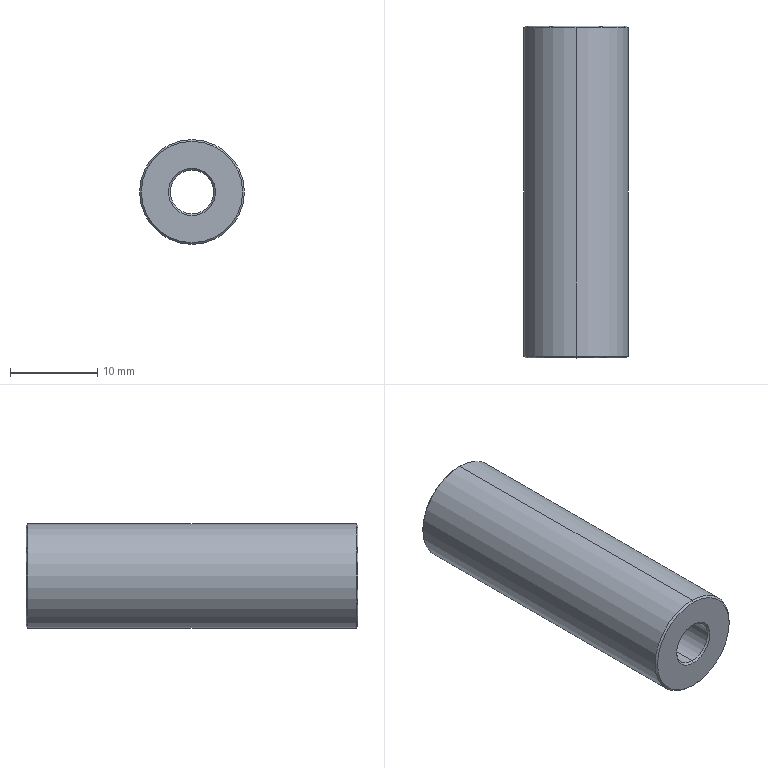Part | STEP file | NCLA5-12-38 | 1 solid | 14 faces | box 12 x 38 x 12 mm | volume 3549 mm3 | cone 8 | cylinder 4 | plane 2 | commonest cylinder face diameters 5 x2 12 x2
STEP:
#1=CARTESIAN_POINT('',(0.,0.,0.));
#2=DIRECTION('',(0.,0.,1.));
#3=DIRECTION('',(1.,0.,0.));
#4=AXIS2_PLACEMENT_3D('',#1,#2,#3);
#5=CARTESIAN_POINT('',(0.,0.2,-2.5));
#6=VERTEX_POINT('',#5);
#7=CARTESIAN_POINT('',(0.,0.,-2.7));
#8=VERTEX_POINT('',#7);
#9=CARTESIAN_POINT('',(0.,0.2,-2.5));
#10=DIRECTION('',(0.,-0.7071,-0.7071));
#11=VECTOR('',#10,1.);
#12=LINE('',#9,#11);
#13=CARTESIAN_POINT('',(0.,0.2,0.));
#14=DIRECTION('',(0.,-1.,0.));
#15=DIRECTION('',(0.,0.,-1.));
#16=AXIS2_PLACEMENT_3D('',#13,#14,#15);
#17=CONICAL_SURFACE('',#16,2.5,0.7854);
#18=CARTESIAN_POINT('',(6.283,0.));
#19=DIRECTION('',(0.,1.));
#20=VECTOR('',#19,1.);
#21=LINE('',#18,#20);
#22=(GEOMETRIC_REPRESENTATION_CONTEXT(2)PARAMETRIC_REPRESENTATION_CONTEXT()REPRESENTATION_CONTEXT('',''));
#23=DEFINITIONAL_REPRESENTATION('',(#21),#22);
#24=PCURVE('',#17,#23);
#25=CARTESIAN_POINT('',(0.,0.2,0.));
#26=DIRECTION('',(0.,-1.,0.));
#27=DIRECTION('',(0.,0.,-1.));
#28=AXIS2_PLACEMENT_3D('',#25,#26,#27);
#29=CONICAL_SURFACE('',#28,2.5,0.7854);
#30=CARTESIAN_POINT('',(0.,0.));
#31=DIRECTION('',(0.,1.));
#32=VECTOR('',#31,1.);
#33=LINE('',#30,#32);
#34=(GEOMETRIC_REPRESENTATION_CONTEXT(2)PARAMETRIC_REPRESENTATION_CONTEXT()REPRESENTATION_CONTEXT('',''));
#35=DEFINITIONAL_REPRESENTATION('',(#33),#34);
#36=PCURVE('',#29,#35);
#37=SURFACE_CURVE('',#12,(#24,#36),.PCURVE_S1.);
#38=EDGE_CURVE('',#6,#8,#37,.T.);
#39=ORIENTED_EDGE('',*,*,#38,.T.);
#40=CARTESIAN_POINT('',(0.,0.,2.7));
#41=VERTEX_POINT('',#40);
#42=CARTESIAN_POINT('',(0.,0.,0.));
#43=DIRECTION('',(0.,-1.,0.));
#44=DIRECTION('',(0.,0.,-1.));
#45=AXIS2_PLACEMENT_3D('',#42,#43,#44);
#46=CIRCLE('',#45,2.7);
#47=CARTESIAN_POINT('',(0.,0.2));
#48=DIRECTION('',(1.,0.));
#49=VECTOR('',#48,1.);
#50=LINE('',#47,#49);
#51=(GEOMETRIC_REPRESENTATION_CONTEXT(2)PARAMETRIC_REPRESENTATION_CONTEXT()REPRESENTATION_CONTEXT('',''));
#52=DEFINITIONAL_REPRESENTATION('',(#50),#51);
#53=PCURVE('',#17,#52);
#54=CARTESIAN_POINT('',(7.3,0.,0.));
#55=DIRECTION('',(0.,1.,0.));
#56=DIRECTION('',(0.,0.,1.));
#57=AXIS2_PLACEMENT_3D('',#54,#55,#56);
#58=PLANE('',#57);
#59=CARTESIAN_POINT('',(-2.7,-7.3));
#60=CARTESIAN_POINT('',(-2.7,-2.623));
#61=CARTESIAN_POINT('',(1.35,-4.962));
#62=CARTESIAN_POINT('',(5.4,-7.3));
#63=CARTESIAN_POINT('',(1.35,-9.638));
#64=CARTESIAN_POINT('',(-2.7,-11.977));
#65=CARTESIAN_POINT('',(-2.7,-7.3));
#66=(BOUNDED_CURVE()B_SPLINE_CURVE(2,(#59,#60,#61,#62,#63,#64,#65),.UNSPECIFIED.,.T.,.F.)B_SPLINE_CURVE_WITH_KNOTS((1,2,2,2,2,1),(-2.094,0.,2.094,4.189,6.283,8.378),.UNSPECIFIED.)CURVE()GEOMETRIC_REPRESENTATION_ITEM()RATIONAL_B_SPLINE_CURVE((1.,0.5,1.,0.5,1.,0.5,1.))REPRESENTATION_ITEM(''));
#67=(GEOMETRIC_REPRESENTATION_CONTEXT(2)PARAMETRIC_REPRESENTATION_CONTEXT()REPRESENTATION_CONTEXT('',''));
#68=DEFINITIONAL_REPRESENTATION('',(#66),#67);
#69=PCURVE('',#58,#68);
#70=SURFACE_CURVE('',#46,(#53,#69),.PCURVE_S1.);
#71=EDGE_CURVE('',#41,#8,#70,.T.);
#72=ORIENTED_EDGE('',*,*,#71,.F.);
#73=CARTESIAN_POINT('',(0.,0.2,2.5));
#74=VERTEX_POINT('',#73);
#75=CARTESIAN_POINT('',(0.,0.2,2.5));
#76=DIRECTION('',(0.,-0.7071,0.7071));
#77=VECTOR('',#76,1.);
#78=LINE('',#75,#77);
#79=CARTESIAN_POINT('',(3.142,0.));
#80=DIRECTION('',(0.,1.));
#81=VECTOR('',#80,1.);
#82=LINE('',#79,#81);
#83=(GEOMETRIC_REPRESENTATION_CONTEXT(2)PARAMETRIC_REPRESENTATION_CONTEXT()REPRESENTATION_CONTEXT('',''));
#84=DEFINITIONAL_REPRESENTATION('',(#82),#83);
#85=PCURVE('',#17,#84);
#86=CARTESIAN_POINT('',(3.142,0.));
#87=DIRECTION('',(0.,1.));
#88=VECTOR('',#87,1.);
#89=LINE('',#86,#88);
#90=(GEOMETRIC_REPRESENTATION_CONTEXT(2)PARAMETRIC_REPRESENTATION_CONTEXT()REPRESENTATION_CONTEXT('',''));
#91=DEFINITIONAL_REPRESENTATION('',(#89),#90);
#92=PCURVE('',#29,#91);
#93=SURFACE_CURVE('',#78,(#85,#92),.PCURVE_S1.);
#94=EDGE_CURVE('',#74,#41,#93,.T.);
#95=ORIENTED_EDGE('',*,*,#94,.F.);
#96=CARTESIAN_POINT('',(0.,0.2,0.));
#97=DIRECTION('',(0.,-1.,0.));
#98=DIRECTION('',(0.,0.,-1.));
#99=AXIS2_PLACEMENT_3D('',#96,#97,#98);
#100=CIRCLE('',#99,2.5);
#101=CARTESIAN_POINT('',(0.,0.));
#102=DIRECTION('',(1.,0.));
#103=VECTOR('',#102,1.);
#104=LINE('',#101,#103);
#105=(GEOMETRIC_REPRESENTATION_CONTEXT(2)PARAMETRIC_REPRESENTATION_CONTEXT()REPRESENTATION_CONTEXT('',''));
#106=DEFINITIONAL_REPRESENTATION('',(#104),#105);
#107=PCURVE('',#17,#106);
#108=CARTESIAN_POINT('',(0.,0.,0.));
#109=DIRECTION('',(0.,-1.,0.));
#110=DIRECTION('',(0.,0.,-1.));
#111=AXIS2_PLACEMENT_3D('',#108,#109,#110);
#112=CYLINDRICAL_SURFACE('',#111,2.5);
#113=CARTESIAN_POINT('',(0.,-0.2));
#114=DIRECTION('',(1.,0.));
#115=VECTOR('',#114,1.);
#116=LINE('',#113,#115);
#117=(GEOMETRIC_REPRESENTATION_CONTEXT(2)PARAMETRIC_REPRESENTATION_CONTEXT()REPRESENTATION_CONTEXT('',''));
#118=DEFINITIONAL_REPRESENTATION('',(#116),#117);
#119=PCURVE('',#112,#118);
#120=SURFACE_CURVE('',#100,(#107,#119),.PCURVE_S1.);
#121=EDGE_CURVE('',#74,#6,#120,.T.);
#122=ORIENTED_EDGE('',*,*,#121,.T.);
#123=EDGE_LOOP('',(#39,#72,#95,#122));
#124=FACE_BOUND('',#123,.F.);
#125=ADVANCED_FACE('',(#124),#17,.F.);
#126=CARTESIAN_POINT('',(0.,37.8,-2.5));
#127=VERTEX_POINT('',#126);
#128=CARTESIAN_POINT('',(0.,0.,-2.5));
#129=DIRECTION('',(0.,-1.,0.));
#130=VECTOR('',#129,1.);
#131=LINE('',#128,#130);
#132=CARTESIAN_POINT('',(6.283,0.));
#133=DIRECTION('',(0.,1.));
#134=VECTOR('',#133,1.);
#135=LINE('',#132,#134);
#136=(GEOMETRIC_REPRESENTATION_CONTEXT(2)PARAMETRIC_REPRESENTATION_CONTEXT()REPRESENTATION_CONTEXT('',''));
#137=DEFINITIONAL_REPRESENTATION('',(#135),#136);
#138=PCURVE('',#112,#137);
#139=CARTESIAN_POINT('',(0.,0.,0.));
#140=DIRECTION('',(0.,-1.,0.));
#141=DIRECTION('',(0.,0.,-1.));
#142=AXIS2_PLACEMENT_3D('',#139,#140,#141);
#143=CYLINDRICAL_SURFACE('',#142,2.5);
#144=CARTESIAN_POINT('',(0.,0.));
#145=DIRECTION('',(0.,1.));
#146=VECTOR('',#145,1.);
#147=LINE('',#144,#146);
#148=(GEOMETRIC_REPRESENTATION_CONTEXT(2)PARAMETRIC_REPRESENTATION_CONTEXT()REPRESENTATION_CONTEXT('',''));
#149=DEFINITIONAL_REPRESENTATION('',(#147),#148);
#150=PCURVE('',#143,#149);
#151=SURFACE_CURVE('',#131,(#138,#150),.PCURVE_S1.);
#152=EDGE_CURVE('',#127,#6,#151,.T.);
#153=ORIENTED_EDGE('',*,*,#152,.T.);
#154=ORIENTED_EDGE('',*,*,#121,.F.);
#155=CARTESIAN_POINT('',(0.,37.8,2.5));
#156=VERTEX_POINT('',#155);
#157=CARTESIAN_POINT('',(0.,0.,2.5));
#158=DIRECTION('',(0.,-1.,0.));
#159=VECTOR('',#158,1.);
#160=LINE('',#157,#159);
#161=CARTESIAN_POINT('',(3.142,0.));
#162=DIRECTION('',(0.,1.));
#163=VECTOR('',#162,1.);
#164=LINE('',#161,#163);
#165=(GEOMETRIC_REPRESENTATION_CONTEXT(2)PARAMETRIC_REPRESENTATION_CONTEXT()REPRESENTATION_CONTEXT('',''));
#166=DEFINITIONAL_REPRESENTATION('',(#164),#165);
#167=PCURVE('',#112,#166);
#168=CARTESIAN_POINT('',(3.142,0.));
#169=DIRECTION('',(0.,1.));
#170=VECTOR('',#169,1.);
#171=LINE('',#168,#170);
#172=(GEOMETRIC_REPRESENTATION_CONTEXT(2)PARAMETRIC_REPRESENTATION_CONTEXT()REPRESENTATION_CONTEXT('',''));
#173=DEFINITIONAL_REPRESENTATION('',(#171),#172);
#174=PCURVE('',#143,#173);
#175=SURFACE_CURVE('',#160,(#167,#174),.PCURVE_S1.);
#176=EDGE_CURVE('',#156,#74,#175,.T.);
#177=ORIENTED_EDGE('',*,*,#176,.F.);
#178=CARTESIAN_POINT('',(0.,37.8,0.));
#179=DIRECTION('',(0.,-1.,0.));
#180=DIRECTION('',(0.,0.,-1.));
#181=AXIS2_PLACEMENT_3D('',#178,#179,#180);
#182=CIRCLE('',#181,2.5);
#183=CARTESIAN_POINT('',(0.,-37.8));
#184=DIRECTION('',(1.,0.));
#185=VECTOR('',#184,1.);
#186=LINE('',#183,#185);
#187=(GEOMETRIC_REPRESENTATION_CONTEXT(2)PARAMETRIC_REPRESENTATION_CONTEXT()REPRESENTATION_CONTEXT('',''));
#188=DEFINITIONAL_REPRESENTATION('',(#186),#187);
#189=PCURVE('',#112,#188);
#190=CARTESIAN_POINT('',(0.,38.,0.));
#191=DIRECTION('',(0.,1.,0.));
#192=DIRECTION('',(0.,0.,1.));
#193=AXIS2_PLACEMENT_3D('',#190,#191,#192);
#194=CONICAL_SURFACE('',#193,2.7,0.7854);
#195=CARTESIAN_POINT('',(9.425,-0.2));
#196=DIRECTION('',(-1.,0.));
#197=VECTOR('',#196,1.);
#198=LINE('',#195,#197);
#199=(GEOMETRIC_REPRESENTATION_CONTEXT(2)PARAMETRIC_REPRESENTATION_CONTEXT()REPRESENTATION_CONTEXT('',''));
#200=DEFINITIONAL_REPRESENTATION('',(#198),#199);
#201=PCURVE('',#194,#200);
#202=SURFACE_CURVE('',#182,(#189,#201),.PCURVE_S1.);
#203=EDGE_CURVE('',#156,#127,#202,.T.);
#204=ORIENTED_EDGE('',*,*,#203,.T.);
#205=EDGE_LOOP('',(#153,#154,#177,#204));
#206=FACE_BOUND('',#205,.F.);
#207=ADVANCED_FACE('',(#206),#112,.F.);
#208=CARTESIAN_POINT('',(0.,38.,2.7));
#209=VERTEX_POINT('',#208);
#210=CARTESIAN_POINT('',(0.,38.,2.7));
#211=DIRECTION('',(0.,0.7071,0.7071));
#212=VECTOR('',#211,1.);
#213=LINE('',#210,#212);
#214=CARTESIAN_POINT('',(6.283,0.));
#215=DIRECTION('',(0.,1.));
#216=VECTOR('',#215,1.);
#217=LINE('',#214,#216);
#218=(GEOMETRIC_REPRESENTATION_CONTEXT(2)PARAMETRIC_REPRESENTATION_CONTEXT()REPRESENTATION_CONTEXT('',''));
#219=DEFINITIONAL_REPRESENTATION('',(#217),#218);
#220=PCURVE('',#194,#219);
#221=CARTESIAN_POINT('',(0.,38.,0.));
#222=DIRECTION('',(0.,1.,0.));
#223=DIRECTION('',(0.,0.,1.));
#224=AXIS2_PLACEMENT_3D('',#221,#222,#223);
#225=CONICAL_SURFACE('',#224,2.7,0.7854);
#226=CARTESIAN_POINT('',(0.,0.));
#227=DIRECTION('',(0.,1.));
#228=VECTOR('',#227,1.);
#229=LINE('',#226,#228);
#230=(GEOMETRIC_REPRESENTATION_CONTEXT(2)PARAMETRIC_REPRESENTATION_CONTEXT()REPRESENTATION_CONTEXT('',''));
#231=DEFINITIONAL_REPRESENTATION('',(#229),#230);
#232=PCURVE('',#225,#231);
#233=SURFACE_CURVE('',#213,(#220,#232),.PCURVE_S1.);
#234=EDGE_CURVE('',#156,#209,#233,.T.);
#235=ORIENTED_EDGE('',*,*,#234,.T.);
#236=CARTESIAN_POINT('',(0.,38.,-2.7));
#237=VERTEX_POINT('',#236);
#238=CARTESIAN_POINT('',(0.,38.,0.));
#239=DIRECTION('',(0.,-1.,0.));
#240=DIRECTION('',(0.,0.,-1.));
#241=AXIS2_PLACEMENT_3D('',#238,#239,#240);
#242=CIRCLE('',#241,2.7);
#243=CARTESIAN_POINT('',(9.425,0.));
#244=DIRECTION('',(-1.,0.));
#245=VECTOR('',#244,1.);
#246=LINE('',#243,#245);
#247=(GEOMETRIC_REPRESENTATION_CONTEXT(2)PARAMETRIC_REPRESENTATION_CONTEXT()REPRESENTATION_CONTEXT('',''));
#248=DEFINITIONAL_REPRESENTATION('',(#246),#247);
#249=PCURVE('',#194,#248);
#250=CARTESIAN_POINT('',(0.,38.,0.));
#251=DIRECTION('',(0.,-1.,0.));
#252=DIRECTION('',(0.,0.,-1.));
#253=AXIS2_PLACEMENT_3D('',#250,#251,#252);
#254=PLANE('',#253);
#255=CARTESIAN_POINT('',(0.,0.));
#256=DIRECTION('',(1.,0.));
#257=AXIS2_PLACEMENT_2D('',#255,#256);
#258=CIRCLE('',#257,2.7);
#259=(GEOMETRIC_REPRESENTATION_CONTEXT(2)PARAMETRIC_REPRESENTATION_CONTEXT()REPRESENTATION_CONTEXT('',''));
#260=DEFINITIONAL_REPRESENTATION('',(#258),#259);
#261=PCURVE('',#254,#260);
#262=SURFACE_CURVE('',#242,(#249,#261),.PCURVE_S1.);
#263=EDGE_CURVE('',#209,#237,#262,.T.);
#264=ORIENTED_EDGE('',*,*,#263,.T.);
#265=CARTESIAN_POINT('',(0.,38.,-2.7));
#266=DIRECTION('',(0.,0.7071,-0.7071));
#267=VECTOR('',#266,1.);
#268=LINE('',#265,#267);
#269=CARTESIAN_POINT('',(3.142,0.));
#270=DIRECTION('',(0.,1.));
#271=VECTOR('',#270,1.);
#272=LINE('',#269,#271);
#273=(GEOMETRIC_REPRESENTATION_CONTEXT(2)PARAMETRIC_REPRESENTATION_CONTEXT()REPRESENTATION_CONTEXT('',''));
#274=DEFINITIONAL_REPRESENTATION('',(#272),#273);
#275=PCURVE('',#194,#274);
#276=CARTESIAN_POINT('',(3.142,0.));
#277=DIRECTION('',(0.,1.));
#278=VECTOR('',#277,1.);
#279=LINE('',#276,#278);
#280=(GEOMETRIC_REPRESENTATION_CONTEXT(2)PARAMETRIC_REPRESENTATION_CONTEXT()REPRESENTATION_CONTEXT('',''));
#281=DEFINITIONAL_REPRESENTATION('',(#279),#280);
#282=PCURVE('',#225,#281);
#283=SURFACE_CURVE('',#268,(#275,#282),.PCURVE_S1.);
#284=EDGE_CURVE('',#127,#237,#283,.T.);
#285=ORIENTED_EDGE('',*,*,#284,.F.);
#286=ORIENTED_EDGE('',*,*,#203,.F.);
#287=EDGE_LOOP('',(#235,#264,#285,#286));
#288=FACE_BOUND('',#287,.F.);
#289=ADVANCED_FACE('',(#288),#194,.F.);
#290=CARTESIAN_POINT('',(0.,0.,-5.8));
#291=VERTEX_POINT('',#290);
#292=CARTESIAN_POINT('',(0.,0.,5.8));
#293=VERTEX_POINT('',#292);
#294=CARTESIAN_POINT('',(0.,0.,0.));
#295=DIRECTION('',(0.,-1.,0.));
#296=DIRECTION('',(0.,0.,1.));
#297=AXIS2_PLACEMENT_3D('',#294,#295,#296);
#298=CIRCLE('',#297,5.8);
#299=CARTESIAN_POINT('',(0.,0.2,0.));
#300=DIRECTION('',(0.,1.,0.));
#301=DIRECTION('',(0.,0.,1.));
#302=AXIS2_PLACEMENT_3D('',#299,#300,#301);
#303=CONICAL_SURFACE('',#302,6.,0.7854);
#304=CARTESIAN_POINT('',(6.283,-0.2));
#305=DIRECTION('',(-1.,0.));
#306=VECTOR('',#305,1.);
#307=LINE('',#304,#306);
#308=(GEOMETRIC_REPRESENTATION_CONTEXT(2)PARAMETRIC_REPRESENTATION_CONTEXT()REPRESENTATION_CONTEXT('',''));
#309=DEFINITIONAL_REPRESENTATION('',(#307),#308);
#310=PCURVE('',#303,#309);
#311=CARTESIAN_POINT('',(5.8,-7.3));
#312=CARTESIAN_POINT('',(5.8,-17.346));
#313=CARTESIAN_POINT('',(-2.9,-12.323));
#314=CARTESIAN_POINT('',(-11.6,-7.3));
#315=CARTESIAN_POINT('',(-2.9,-2.277));
#316=CARTESIAN_POINT('',(5.8,2.746));
#317=CARTESIAN_POINT('',(5.8,-7.3));
#318=(BOUNDED_CURVE()B_SPLINE_CURVE(2,(#311,#312,#313,#314,#315,#316,#317),.UNSPECIFIED.,.T.,.F.)B_SPLINE_CURVE_WITH_KNOTS((1,2,2,2,2,1),(-2.094,0.,2.094,4.189,6.283,8.378),.UNSPECIFIED.)CURVE()GEOMETRIC_REPRESENTATION_ITEM()RATIONAL_B_SPLINE_CURVE((1.,0.5,1.,0.5,1.,0.5,1.))REPRESENTATION_ITEM(''));
#319=(GEOMETRIC_REPRESENTATION_CONTEXT(2)PARAMETRIC_REPRESENTATION_CONTEXT()REPRESENTATION_CONTEXT('',''));
#320=DEFINITIONAL_REPRESENTATION('',(#318),#319);
#321=PCURVE('',#58,#320);
#322=SURFACE_CURVE('',#298,(#310,#321),.PCURVE_S1.);
#323=EDGE_CURVE('',#291,#293,#322,.T.);
#324=ORIENTED_EDGE('',*,*,#323,.F.);
#325=CARTESIAN_POINT('',(0.,0.2,-6.));
#326=VERTEX_POINT('',#325);
#327=CARTESIAN_POINT('',(0.,0.2,-6.));
#328=DIRECTION('',(0.,0.7071,-0.7071));
#329=VECTOR('',#328,1.);
#330=LINE('',#327,#329);
#331=CARTESIAN_POINT('',(3.142,0.));
#332=DIRECTION('',(0.,1.));
#333=VECTOR('',#332,1.);
#334=LINE('',#331,#333);
#335=(GEOMETRIC_REPRESENTATION_CONTEXT(2)PARAMETRIC_REPRESENTATION_CONTEXT()REPRESENTATION_CONTEXT('',''));
#336=DEFINITIONAL_REPRESENTATION('',(#334),#335);
#337=PCURVE('',#303,#336);
#338=CARTESIAN_POINT('',(0.,0.2,0.));
#339=DIRECTION('',(0.,1.,0.));
#340=DIRECTION('',(0.,0.,1.));
#341=AXIS2_PLACEMENT_3D('',#338,#339,#340);
#342=CONICAL_SURFACE('',#341,6.,0.7854);
#343=CARTESIAN_POINT('',(3.142,0.));
#344=DIRECTION('',(0.,1.));
#345=VECTOR('',#344,1.);
#346=LINE('',#343,#345);
#347=(GEOMETRIC_REPRESENTATION_CONTEXT(2)PARAMETRIC_REPRESENTATION_CONTEXT()REPRESENTATION_CONTEXT('',''));
#348=DEFINITIONAL_REPRESENTATION('',(#346),#347);
#349=PCURVE('',#342,#348);
#350=SURFACE_CURVE('',#330,(#337,#349),.PCURVE_S1.);
#351=EDGE_CURVE('',#291,#326,#350,.T.);
#352=ORIENTED_EDGE('',*,*,#351,.T.);
#353=CARTESIAN_POINT('',(0.,0.2,6.));
#354=VERTEX_POINT('',#353);
#355=CARTESIAN_POINT('',(0.,0.2,0.));
#356=DIRECTION('',(0.,-1.,0.));
#357=DIRECTION('',(0.,0.,1.));
#358=AXIS2_PLACEMENT_3D('',#355,#356,#357);
#359=CIRCLE('',#358,6.);
#360=CARTESIAN_POINT('',(6.283,0.));
#361=DIRECTION('',(-1.,0.));
#362=VECTOR('',#361,1.);
#363=LINE('',#360,#362);
#364=(GEOMETRIC_REPRESENTATION_CONTEXT(2)PARAMETRIC_REPRESENTATION_CONTEXT()REPRESENTATION_CONTEXT('',''));
#365=DEFINITIONAL_REPRESENTATION('',(#363),#364);
#366=PCURVE('',#303,#365);
#367=CARTESIAN_POINT('',(0.,0.,0.));
#368=DIRECTION('',(0.,-1.,0.));
#369=DIRECTION('',(0.,0.,-1.));
#370=AXIS2_PLACEMENT_3D('',#367,#368,#369);
#371=CYLINDRICAL_SURFACE('',#370,6.);
#372=CARTESIAN_POINT('',(-3.142,-0.2));
#373=DIRECTION('',(1.,0.));
#374=VECTOR('',#373,1.);
#375=LINE('',#372,#374);
#376=(GEOMETRIC_REPRESENTATION_CONTEXT(2)PARAMETRIC_REPRESENTATION_CONTEXT()REPRESENTATION_CONTEXT('',''));
#377=DEFINITIONAL_REPRESENTATION('',(#375),#376);
#378=PCURVE('',#371,#377);
#379=SURFACE_CURVE('',#359,(#366,#378),.PCURVE_S1.);
#380=EDGE_CURVE('',#326,#354,#379,.T.);
#381=ORIENTED_EDGE('',*,*,#380,.T.);
#382=CARTESIAN_POINT('',(0.,0.2,6.));
#383=DIRECTION('',(0.,0.7071,0.7071));
#384=VECTOR('',#383,1.);
#385=LINE('',#382,#384);
#386=CARTESIAN_POINT('',(0.,0.));
#387=DIRECTION('',(0.,1.));
#388=VECTOR('',#387,1.);
#389=LINE('',#386,#388);
#390=(GEOMETRIC_REPRESENTATION_CONTEXT(2)PARAMETRIC_REPRESENTATION_CONTEXT()REPRESENTATION_CONTEXT('',''));
#391=DEFINITIONAL_REPRESENTATION('',(#389),#390);
#392=PCURVE('',#303,#391);
#393=CARTESIAN_POINT('',(6.283,0.));
#394=DIRECTION('',(0.,1.));
#395=VECTOR('',#394,1.);
#396=LINE('',#393,#395);
#397=(GEOMETRIC_REPRESENTATION_CONTEXT(2)PARAMETRIC_REPRESENTATION_CONTEXT()REPRESENTATION_CONTEXT('',''));
#398=DEFINITIONAL_REPRESENTATION('',(#396),#397);
#399=PCURVE('',#342,#398);
#400=SURFACE_CURVE('',#385,(#392,#399),.PCURVE_S1.);
#401=EDGE_CURVE('',#293,#354,#400,.T.);
#402=ORIENTED_EDGE('',*,*,#401,.F.);
#403=EDGE_LOOP('',(#324,#352,#381,#402));
#404=FACE_BOUND('',#403,.T.);
#405=ADVANCED_FACE('',(#404),#303,.T.);
#406=CARTESIAN_POINT('',(0.,37.8,-6.));
#407=VERTEX_POINT('',#406);
#408=CARTESIAN_POINT('',(0.,37.8,6.));
#409=VERTEX_POINT('',#408);
#410=CARTESIAN_POINT('',(0.,37.8,0.));
#411=DIRECTION('',(0.,-1.,0.));
#412=DIRECTION('',(0.,0.,-1.));
#413=AXIS2_PLACEMENT_3D('',#410,#411,#412);
#414=CIRCLE('',#413,6.);
#415=CARTESIAN_POINT('',(0.,-37.8));
#416=DIRECTION('',(1.,0.));
#417=VECTOR('',#416,1.);
#418=LINE('',#415,#417);
#419=(GEOMETRIC_REPRESENTATION_CONTEXT(2)PARAMETRIC_REPRESENTATION_CONTEXT()REPRESENTATION_CONTEXT('',''));
#420=DEFINITIONAL_REPRESENTATION('',(#418),#419);
#421=PCURVE('',#371,#420);
#422=CARTESIAN_POINT('',(0.,38.,0.));
#423=DIRECTION('',(0.,-1.,0.));
#424=DIRECTION('',(0.,0.,-1.));
#425=AXIS2_PLACEMENT_3D('',#422,#423,#424);
#426=CONICAL_SURFACE('',#425,5.8,0.7854);
#427=CARTESIAN_POINT('',(0.,0.2));
#428=DIRECTION('',(1.,0.));
#429=VECTOR('',#428,1.);
#430=LINE('',#427,#429);
#431=(GEOMETRIC_REPRESENTATION_CONTEXT(2)PARAMETRIC_REPRESENTATION_CONTEXT()REPRESENTATION_CONTEXT('',''));
#432=DEFINITIONAL_REPRESENTATION('',(#430),#431);
#433=PCURVE('',#426,#432);
#434=SURFACE_CURVE('',#414,(#421,#433),.PCURVE_S1.);
#435=EDGE_CURVE('',#407,#409,#434,.T.);
#436=ORIENTED_EDGE('',*,*,#435,.T.);
#437=CARTESIAN_POINT('',(0.,0.,6.));
#438=DIRECTION('',(0.,-1.,0.));
#439=VECTOR('',#438,1.);
#440=LINE('',#437,#439);
#441=CARTESIAN_POINT('',(3.142,0.));
#442=DIRECTION('',(0.,1.));
#443=VECTOR('',#442,1.);
#444=LINE('',#441,#443);
#445=(GEOMETRIC_REPRESENTATION_CONTEXT(2)PARAMETRIC_REPRESENTATION_CONTEXT()REPRESENTATION_CONTEXT('',''));
#446=DEFINITIONAL_REPRESENTATION('',(#444),#445);
#447=PCURVE('',#371,#446);
#448=CARTESIAN_POINT('',(0.,0.,0.));
#449=DIRECTION('',(0.,-1.,0.));
#450=DIRECTION('',(0.,0.,-1.));
#451=AXIS2_PLACEMENT_3D('',#448,#449,#450);
#452=CYLINDRICAL_SURFACE('',#451,6.);
#453=CARTESIAN_POINT('',(3.142,0.));
#454=DIRECTION('',(0.,1.));
#455=VECTOR('',#454,1.);
#456=LINE('',#453,#455);
#457=(GEOMETRIC_REPRESENTATION_CONTEXT(2)PARAMETRIC_REPRESENTATION_CONTEXT()REPRESENTATION_CONTEXT('',''));
#458=DEFINITIONAL_REPRESENTATION('',(#456),#457);
#459=PCURVE('',#452,#458);
#460=SURFACE_CURVE('',#440,(#447,#459),.PCURVE_S1.);
#461=EDGE_CURVE('',#409,#354,#460,.T.);
#462=ORIENTED_EDGE('',*,*,#461,.T.);
#463=ORIENTED_EDGE('',*,*,#380,.F.);
#464=CARTESIAN_POINT('',(0.,0.,-6.));
#465=DIRECTION('',(0.,-1.,0.));
#466=VECTOR('',#465,1.);
#467=LINE('',#464,#466);
#468=CARTESIAN_POINT('',(0.,0.));
#469=DIRECTION('',(0.,1.));
#470=VECTOR('',#469,1.);
#471=LINE('',#468,#470);
#472=(GEOMETRIC_REPRESENTATION_CONTEXT(2)PARAMETRIC_REPRESENTATION_CONTEXT()REPRESENTATION_CONTEXT('',''));
#473=DEFINITIONAL_REPRESENTATION('',(#471),#472);
#474=PCURVE('',#371,#473);
#475=CARTESIAN_POINT('',(6.283,0.));
#476=DIRECTION('',(0.,1.));
#477=VECTOR('',#476,1.);
#478=LINE('',#475,#477);
#479=(GEOMETRIC_REPRESENTATION_CONTEXT(2)PARAMETRIC_REPRESENTATION_CONTEXT()REPRESENTATION_CONTEXT('',''));
#480=DEFINITIONAL_REPRESENTATION('',(#478),#479);
#481=PCURVE('',#452,#480);
#482=SURFACE_CURVE('',#467,(#474,#481),.PCURVE_S1.);
#483=EDGE_CURVE('',#407,#326,#482,.T.);
#484=ORIENTED_EDGE('',*,*,#483,.F.);
#485=EDGE_LOOP('',(#436,#462,#463,#484));
#486=FACE_BOUND('',#485,.T.);
#487=ADVANCED_FACE('',(#486),#371,.T.);
#488=CARTESIAN_POINT('',(0.,38.,-5.8));
#489=VERTEX_POINT('',#488);
#490=CARTESIAN_POINT('',(0.,38.,5.8));
#491=VERTEX_POINT('',#490);
#492=CARTESIAN_POINT('',(0.,38.,0.));
#493=DIRECTION('',(0.,-1.,0.));
#494=DIRECTION('',(0.,0.,-1.));
#495=AXIS2_PLACEMENT_3D('',#492,#493,#494);
#496=CIRCLE('',#495,5.8);
#497=CARTESIAN_POINT('',(0.,0.));
#498=DIRECTION('',(1.,0.));
#499=VECTOR('',#498,1.);
#500=LINE('',#497,#499);
#501=(GEOMETRIC_REPRESENTATION_CONTEXT(2)PARAMETRIC_REPRESENTATION_CONTEXT()REPRESENTATION_CONTEXT('',''));
#502=DEFINITIONAL_REPRESENTATION('',(#500),#501);
#503=PCURVE('',#426,#502);
#504=CARTESIAN_POINT('',(0.,0.));
#505=DIRECTION('',(1.,0.));
#506=AXIS2_PLACEMENT_2D('',#504,#505);
#507=CIRCLE('',#506,5.8);
#508=(GEOMETRIC_REPRESENTATION_CONTEXT(2)PARAMETRIC_REPRESENTATION_CONTEXT()REPRESENTATION_CONTEXT('',''));
#509=DEFINITIONAL_REPRESENTATION('',(#507),#508);
#510=PCURVE('',#254,#509);
#511=SURFACE_CURVE('',#496,(#503,#510),.PCURVE_S1.);
#512=EDGE_CURVE('',#489,#491,#511,.T.);
#513=ORIENTED_EDGE('',*,*,#512,.T.);
#514=CARTESIAN_POINT('',(0.,38.,5.8));
#515=DIRECTION('',(0.,-0.7071,0.7071));
#516=VECTOR('',#515,1.);
#517=LINE('',#514,#516);
#518=CARTESIAN_POINT('',(3.142,0.));
#519=DIRECTION('',(0.,1.));
#520=VECTOR('',#519,1.);
#521=LINE('',#518,#520);
#522=(GEOMETRIC_REPRESENTATION_CONTEXT(2)PARAMETRIC_REPRESENTATION_CONTEXT()REPRESENTATION_CONTEXT('',''));
#523=DEFINITIONAL_REPRESENTATION('',(#521),#522);
#524=PCURVE('',#426,#523);
#525=CARTESIAN_POINT('',(0.,38.,0.));
#526=DIRECTION('',(0.,-1.,0.));
#527=DIRECTION('',(0.,0.,-1.));
#528=AXIS2_PLACEMENT_3D('',#525,#526,#527);
#529=CONICAL_SURFACE('',#528,5.8,0.7854);
#530=CARTESIAN_POINT('',(3.142,0.));
#531=DIRECTION('',(0.,1.));
#532=VECTOR('',#531,1.);
#533=LINE('',#530,#532);
#534=(GEOMETRIC_REPRESENTATION_CONTEXT(2)PARAMETRIC_REPRESENTATION_CONTEXT()REPRESENTATION_CONTEXT('',''));
#535=DEFINITIONAL_REPRESENTATION('',(#533),#534);
#536=PCURVE('',#529,#535);
#537=SURFACE_CURVE('',#517,(#524,#536),.PCURVE_S1.);
#538=EDGE_CURVE('',#491,#409,#537,.T.);
#539=ORIENTED_EDGE('',*,*,#538,.T.);
#540=ORIENTED_EDGE('',*,*,#435,.F.);
#541=CARTESIAN_POINT('',(0.,38.,-5.8));
#542=DIRECTION('',(0.,-0.7071,-0.7071));
#543=VECTOR('',#542,1.);
#544=LINE('',#541,#543);
#545=CARTESIAN_POINT('',(0.,0.));
#546=DIRECTION('',(0.,1.));
#547=VECTOR('',#546,1.);
#548=LINE('',#545,#547);
#549=(GEOMETRIC_REPRESENTATION_CONTEXT(2)PARAMETRIC_REPRESENTATION_CONTEXT()REPRESENTATION_CONTEXT('',''));
#550=DEFINITIONAL_REPRESENTATION('',(#548),#549);
#551=PCURVE('',#426,#550);
#552=CARTESIAN_POINT('',(6.283,0.));
#553=DIRECTION('',(0.,1.));
#554=VECTOR('',#553,1.);
#555=LINE('',#552,#554);
#556=(GEOMETRIC_REPRESENTATION_CONTEXT(2)PARAMETRIC_REPRESENTATION_CONTEXT()REPRESENTATION_CONTEXT('',''));
#557=DEFINITIONAL_REPRESENTATION('',(#555),#556);
#558=PCURVE('',#529,#557);
#559=SURFACE_CURVE('',#544,(#551,#558),.PCURVE_S1.);
#560=EDGE_CURVE('',#489,#407,#559,.T.);
#561=ORIENTED_EDGE('',*,*,#560,.F.);
#562=EDGE_LOOP('',(#513,#539,#540,#561));
#563=FACE_BOUND('',#562,.T.);
#564=ADVANCED_FACE('',(#563),#426,.T.);
#565=ORIENTED_EDGE('',*,*,#512,.F.);
#566=CARTESIAN_POINT('',(0.,38.,0.));
#567=DIRECTION('',(0.,-1.,0.));
#568=DIRECTION('',(0.,0.,-1.));
#569=AXIS2_PLACEMENT_3D('',#566,#567,#568);
#570=CIRCLE('',#569,5.8);
#571=CARTESIAN_POINT('',(0.,0.));
#572=DIRECTION('',(1.,0.));
#573=AXIS2_PLACEMENT_2D('',#571,#572);
#574=CIRCLE('',#573,5.8);
#575=(GEOMETRIC_REPRESENTATION_CONTEXT(2)PARAMETRIC_REPRESENTATION_CONTEXT()REPRESENTATION_CONTEXT('',''));
#576=DEFINITIONAL_REPRESENTATION('',(#574),#575);
#577=PCURVE('',#254,#576);
#578=CARTESIAN_POINT('',(0.,0.));
#579=DIRECTION('',(1.,0.));
#580=VECTOR('',#579,1.);
#581=LINE('',#578,#580);
#582=(GEOMETRIC_REPRESENTATION_CONTEXT(2)PARAMETRIC_REPRESENTATION_CONTEXT()REPRESENTATION_CONTEXT('',''));
#583=DEFINITIONAL_REPRESENTATION('',(#581),#582);
#584=PCURVE('',#529,#583);
#585=SURFACE_CURVE('',#570,(#577,#584),.PCURVE_S1.);
#586=EDGE_CURVE('',#491,#489,#585,.T.);
#587=ORIENTED_EDGE('',*,*,#586,.F.);
#588=EDGE_LOOP('',(#565,#587));
#589=FACE_BOUND('',#588,.T.);
#590=ORIENTED_EDGE('',*,*,#263,.T.);
#591=CARTESIAN_POINT('',(0.,38.,0.));
#592=DIRECTION('',(0.,-1.,0.));
#593=DIRECTION('',(0.,0.,-1.));
#594=AXIS2_PLACEMENT_3D('',#591,#592,#593);
#595=CIRCLE('',#594,2.7);
#596=CARTESIAN_POINT('',(0.,0.));
#597=DIRECTION('',(1.,0.));
#598=AXIS2_PLACEMENT_2D('',#596,#597);
#599=CIRCLE('',#598,2.7);
#600=(GEOMETRIC_REPRESENTATION_CONTEXT(2)PARAMETRIC_REPRESENTATION_CONTEXT()REPRESENTATION_CONTEXT('',''));
#601=DEFINITIONAL_REPRESENTATION('',(#599),#600);
#602=PCURVE('',#254,#601);
#603=CARTESIAN_POINT('',(3.142,0.));
#604=DIRECTION('',(-1.,0.));
#605=VECTOR('',#604,1.);
#606=LINE('',#603,#605);
#607=(GEOMETRIC_REPRESENTATION_CONTEXT(2)PARAMETRIC_REPRESENTATION_CONTEXT()REPRESENTATION_CONTEXT('',''));
#608=DEFINITIONAL_REPRESENTATION('',(#606),#607);
#609=PCURVE('',#225,#608);
#610=SURFACE_CURVE('',#595,(#602,#609),.PCURVE_S1.);
#611=EDGE_CURVE('',#237,#209,#610,.T.);
#612=ORIENTED_EDGE('',*,*,#611,.T.);
#613=EDGE_LOOP('',(#590,#612));
#614=FACE_BOUND('',#613,.T.);
#615=ADVANCED_FACE('',(#589,#614),#254,.F.);
#616=ORIENTED_EDGE('',*,*,#538,.F.);
#617=ORIENTED_EDGE('',*,*,#586,.T.);
#618=ORIENTED_EDGE('',*,*,#560,.T.);
#619=CARTESIAN_POINT('',(0.,37.8,0.));
#620=DIRECTION('',(0.,-1.,0.));
#621=DIRECTION('',(0.,0.,-1.));
#622=AXIS2_PLACEMENT_3D('',#619,#620,#621);
#623=CIRCLE('',#622,6.);
#624=CARTESIAN_POINT('',(0.,0.2));
#625=DIRECTION('',(1.,0.));
#626=VECTOR('',#625,1.);
#627=LINE('',#624,#626);
#628=(GEOMETRIC_REPRESENTATION_CONTEXT(2)PARAMETRIC_REPRESENTATION_CONTEXT()REPRESENTATION_CONTEXT('',''));
#629=DEFINITIONAL_REPRESENTATION('',(#627),#628);
#630=PCURVE('',#529,#629);
#631=CARTESIAN_POINT('',(0.,-37.8));
#632=DIRECTION('',(1.,0.));
#633=VECTOR('',#632,1.);
#634=LINE('',#631,#633);
#635=(GEOMETRIC_REPRESENTATION_CONTEXT(2)PARAMETRIC_REPRESENTATION_CONTEXT()REPRESENTATION_CONTEXT('',''));
#636=DEFINITIONAL_REPRESENTATION('',(#634),#635);
#637=PCURVE('',#452,#636);
#638=SURFACE_CURVE('',#623,(#630,#637),.PCURVE_S1.);
#639=EDGE_CURVE('',#409,#407,#638,.T.);
#640=ORIENTED_EDGE('',*,*,#639,.F.);
#641=EDGE_LOOP('',(#616,#617,#618,#640));
#642=FACE_BOUND('',#641,.T.);
#643=ADVANCED_FACE('',(#642),#529,.T.);
#644=ORIENTED_EDGE('',*,*,#461,.F.);
#645=ORIENTED_EDGE('',*,*,#639,.T.);
#646=ORIENTED_EDGE('',*,*,#483,.T.);
#647=CARTESIAN_POINT('',(0.,0.2,0.));
#648=DIRECTION('',(0.,-1.,0.));
#649=DIRECTION('',(0.,0.,1.));
#650=AXIS2_PLACEMENT_3D('',#647,#648,#649);
#651=CIRCLE('',#650,6.);
#652=CARTESIAN_POINT('',(3.142,-0.2));
#653=DIRECTION('',(1.,0.));
#654=VECTOR('',#653,1.);
#655=LINE('',#652,#654);
#656=(GEOMETRIC_REPRESENTATION_CONTEXT(2)PARAMETRIC_REPRESENTATION_CONTEXT()REPRESENTATION_CONTEXT('',''));
#657=DEFINITIONAL_REPRESENTATION('',(#655),#656);
#658=PCURVE('',#452,#657);
#659=CARTESIAN_POINT('',(6.283,0.));
#660=DIRECTION('',(-1.,0.));
#661=VECTOR('',#660,1.);
#662=LINE('',#659,#661);
#663=(GEOMETRIC_REPRESENTATION_CONTEXT(2)PARAMETRIC_REPRESENTATION_CONTEXT()REPRESENTATION_CONTEXT('',''));
#664=DEFINITIONAL_REPRESENTATION('',(#662),#663);
#665=PCURVE('',#342,#664);
#666=SURFACE_CURVE('',#651,(#658,#665),.PCURVE_S1.);
#667=EDGE_CURVE('',#354,#326,#666,.T.);
#668=ORIENTED_EDGE('',*,*,#667,.F.);
#669=EDGE_LOOP('',(#644,#645,#646,#668));
#670=FACE_BOUND('',#669,.T.);
#671=ADVANCED_FACE('',(#670),#452,.T.);
#672=ORIENTED_EDGE('',*,*,#351,.F.);
#673=CARTESIAN_POINT('',(0.,0.,0.));
#674=DIRECTION('',(0.,-1.,0.));
#675=DIRECTION('',(0.,0.,1.));
#676=AXIS2_PLACEMENT_3D('',#673,#674,#675);
#677=CIRCLE('',#676,5.8);
#678=CARTESIAN_POINT('',(6.283,-0.2));
#679=DIRECTION('',(-1.,0.));
#680=VECTOR('',#679,1.);
#681=LINE('',#678,#680);
#682=(GEOMETRIC_REPRESENTATION_CONTEXT(2)PARAMETRIC_REPRESENTATION_CONTEXT()REPRESENTATION_CONTEXT('',''));
#683=DEFINITIONAL_REPRESENTATION('',(#681),#682);
#684=PCURVE('',#342,#683);
#685=CARTESIAN_POINT('',(5.8,-7.3));
#686=CARTESIAN_POINT('',(5.8,-17.346));
#687=CARTESIAN_POINT('',(-2.9,-12.323));
#688=CARTESIAN_POINT('',(-11.6,-7.3));
#689=CARTESIAN_POINT('',(-2.9,-2.277));
#690=CARTESIAN_POINT('',(5.8,2.746));
#691=CARTESIAN_POINT('',(5.8,-7.3));
#692=(BOUNDED_CURVE()B_SPLINE_CURVE(2,(#685,#686,#687,#688,#689,#690,#691),.UNSPECIFIED.,.T.,.F.)B_SPLINE_CURVE_WITH_KNOTS((1,2,2,2,2,1),(-2.094,0.,2.094,4.189,6.283,8.378),.UNSPECIFIED.)CURVE()GEOMETRIC_REPRESENTATION_ITEM()RATIONAL_B_SPLINE_CURVE((1.,0.5,1.,0.5,1.,0.5,1.))REPRESENTATION_ITEM(''));
#693=(GEOMETRIC_REPRESENTATION_CONTEXT(2)PARAMETRIC_REPRESENTATION_CONTEXT()REPRESENTATION_CONTEXT('',''));
#694=DEFINITIONAL_REPRESENTATION('',(#692),#693);
#695=PCURVE('',#58,#694);
#696=SURFACE_CURVE('',#677,(#684,#695),.PCURVE_S1.);
#697=EDGE_CURVE('',#293,#291,#696,.T.);
#698=ORIENTED_EDGE('',*,*,#697,.F.);
#699=ORIENTED_EDGE('',*,*,#401,.T.);
#700=ORIENTED_EDGE('',*,*,#667,.T.);
#701=EDGE_LOOP('',(#672,#698,#699,#700));
#702=FACE_BOUND('',#701,.T.);
#703=ADVANCED_FACE('',(#702),#342,.T.);
#704=CARTESIAN_POINT('',(0.,0.,0.));
#705=DIRECTION('',(0.,-1.,0.));
#706=DIRECTION('',(0.,0.,-1.));
#707=AXIS2_PLACEMENT_3D('',#704,#705,#706);
#708=CIRCLE('',#707,2.7);
#709=CARTESIAN_POINT('',(-2.7,-7.3));
#710=CARTESIAN_POINT('',(-2.7,-2.623));
#711=CARTESIAN_POINT('',(1.35,-4.962));
#712=CARTESIAN_POINT('',(5.4,-7.3));
#713=CARTESIAN_POINT('',(1.35,-9.638));
#714=CARTESIAN_POINT('',(-2.7,-11.977));
#715=CARTESIAN_POINT('',(-2.7,-7.3));
#716=(BOUNDED_CURVE()B_SPLINE_CURVE(2,(#709,#710,#711,#712,#713,#714,#715),.UNSPECIFIED.,.T.,.F.)B_SPLINE_CURVE_WITH_KNOTS((1,2,2,2,2,1),(-2.094,0.,2.094,4.189,6.283,8.378),.UNSPECIFIED.)CURVE()GEOMETRIC_REPRESENTATION_ITEM()RATIONAL_B_SPLINE_CURVE((1.,0.5,1.,0.5,1.,0.5,1.))REPRESENTATION_ITEM(''));
#717=(GEOMETRIC_REPRESENTATION_CONTEXT(2)PARAMETRIC_REPRESENTATION_CONTEXT()REPRESENTATION_CONTEXT('',''));
#718=DEFINITIONAL_REPRESENTATION('',(#716),#717);
#719=PCURVE('',#58,#718);
#720=CARTESIAN_POINT('',(0.,0.2));
#721=DIRECTION('',(1.,0.));
#722=VECTOR('',#721,1.);
#723=LINE('',#720,#722);
#724=(GEOMETRIC_REPRESENTATION_CONTEXT(2)PARAMETRIC_REPRESENTATION_CONTEXT()REPRESENTATION_CONTEXT('',''));
#725=DEFINITIONAL_REPRESENTATION('',(#723),#724);
#726=PCURVE('',#29,#725);
#727=SURFACE_CURVE('',#708,(#719,#726),.PCURVE_S1.);
#728=EDGE_CURVE('',#8,#41,#727,.T.);
#729=ORIENTED_EDGE('',*,*,#728,.F.);
#730=ORIENTED_EDGE('',*,*,#71,.F.);
#731=EDGE_LOOP('',(#729,#730));
#732=FACE_BOUND('',#731,.T.);
#733=ORIENTED_EDGE('',*,*,#697,.T.);
#734=ORIENTED_EDGE('',*,*,#323,.T.);
#735=EDGE_LOOP('',(#733,#734));
#736=FACE_BOUND('',#735,.T.);
#737=ADVANCED_FACE('',(#732,#736),#58,.F.);
#738=ORIENTED_EDGE('',*,*,#611,.T.);
#739=ORIENTED_EDGE('',*,*,#234,.F.);
#740=CARTESIAN_POINT('',(0.,37.8,0.));
#741=DIRECTION('',(0.,-1.,0.));
#742=DIRECTION('',(0.,0.,-1.));
#743=AXIS2_PLACEMENT_3D('',#740,#741,#742);
#744=CIRCLE('',#743,2.5);
#745=CARTESIAN_POINT('',(3.142,-0.2));
#746=DIRECTION('',(-1.,0.));
#747=VECTOR('',#746,1.);
#748=LINE('',#745,#747);
#749=(GEOMETRIC_REPRESENTATION_CONTEXT(2)PARAMETRIC_REPRESENTATION_CONTEXT()REPRESENTATION_CONTEXT('',''));
#750=DEFINITIONAL_REPRESENTATION('',(#748),#749);
#751=PCURVE('',#225,#750);
#752=CARTESIAN_POINT('',(0.,-37.8));
#753=DIRECTION('',(1.,0.));
#754=VECTOR('',#753,1.);
#755=LINE('',#752,#754);
#756=(GEOMETRIC_REPRESENTATION_CONTEXT(2)PARAMETRIC_REPRESENTATION_CONTEXT()REPRESENTATION_CONTEXT('',''));
#757=DEFINITIONAL_REPRESENTATION('',(#755),#756);
#758=PCURVE('',#143,#757);
#759=SURFACE_CURVE('',#744,(#751,#758),.PCURVE_S1.);
#760=EDGE_CURVE('',#127,#156,#759,.T.);
#761=ORIENTED_EDGE('',*,*,#760,.F.);
#762=ORIENTED_EDGE('',*,*,#284,.T.);
#763=EDGE_LOOP('',(#738,#739,#761,#762));
#764=FACE_BOUND('',#763,.F.);
#765=ADVANCED_FACE('',(#764),#225,.F.);
#766=CARTESIAN_POINT('',(0.,0.2,0.));
#767=DIRECTION('',(0.,-1.,0.));
#768=DIRECTION('',(0.,0.,-1.));
#769=AXIS2_PLACEMENT_3D('',#766,#767,#768);
#770=CIRCLE('',#769,2.5);
#771=CARTESIAN_POINT('',(0.,-0.2));
#772=DIRECTION('',(1.,0.));
#773=VECTOR('',#772,1.);
#774=LINE('',#771,#773);
#775=(GEOMETRIC_REPRESENTATION_CONTEXT(2)PARAMETRIC_REPRESENTATION_CONTEXT()REPRESENTATION_CONTEXT('',''));
#776=DEFINITIONAL_REPRESENTATION('',(#774),#775);
#777=PCURVE('',#143,#776);
#778=CARTESIAN_POINT('',(0.,0.));
#779=DIRECTION('',(1.,0.));
#780=VECTOR('',#779,1.);
#781=LINE('',#778,#780);
#782=(GEOMETRIC_REPRESENTATION_CONTEXT(2)PARAMETRIC_REPRESENTATION_CONTEXT()REPRESENTATION_CONTEXT('',''));
#783=DEFINITIONAL_REPRESENTATION('',(#781),#782);
#784=PCURVE('',#29,#783);
#785=SURFACE_CURVE('',#770,(#777,#784),.PCURVE_S1.);
#786=EDGE_CURVE('',#6,#74,#785,.T.);
#787=ORIENTED_EDGE('',*,*,#786,.F.);
#788=ORIENTED_EDGE('',*,*,#152,.F.);
#789=ORIENTED_EDGE('',*,*,#760,.T.);
#790=ORIENTED_EDGE('',*,*,#176,.T.);
#791=EDGE_LOOP('',(#787,#788,#789,#790));
#792=FACE_BOUND('',#791,.F.);
#793=ADVANCED_FACE('',(#792),#143,.F.);
#794=ORIENTED_EDGE('',*,*,#728,.F.);
#795=ORIENTED_EDGE('',*,*,#38,.F.);
#796=ORIENTED_EDGE('',*,*,#786,.T.);
#797=ORIENTED_EDGE('',*,*,#94,.T.);
#798=EDGE_LOOP('',(#794,#795,#796,#797));
#799=FACE_BOUND('',#798,.F.);
#800=ADVANCED_FACE('',(#799),#29,.F.);
#801=CLOSED_SHELL('',(#125,#207,#289,#405,#487,#564,#615,#643,#671,#703,#737,#765,#793,#800));
#802=MANIFOLD_SOLID_BREP('',#801);
#803=(LENGTH_UNIT()NAMED_UNIT(*)SI_UNIT(.MILLI.,.METRE.));
#804=UNCERTAINTY_MEASURE_WITH_UNIT(LENGTH_MEASURE(0.0000001),#803,'','');
#805=(NAMED_UNIT(*)PLANE_ANGLE_UNIT()SI_UNIT($,.RADIAN.));
#806=(NAMED_UNIT(*)SI_UNIT($,.STERADIAN.)SOLID_ANGLE_UNIT());
#807=(GEOMETRIC_REPRESENTATION_CONTEXT(3)GLOBAL_UNCERTAINTY_ASSIGNED_CONTEXT((#804))GLOBAL_UNIT_ASSIGNED_CONTEXT((#803,#805,#806))REPRESENTATION_CONTEXT('',''));
#808=ADVANCED_BREP_SHAPE_REPRESENTATION('',(#4,#802),#807);